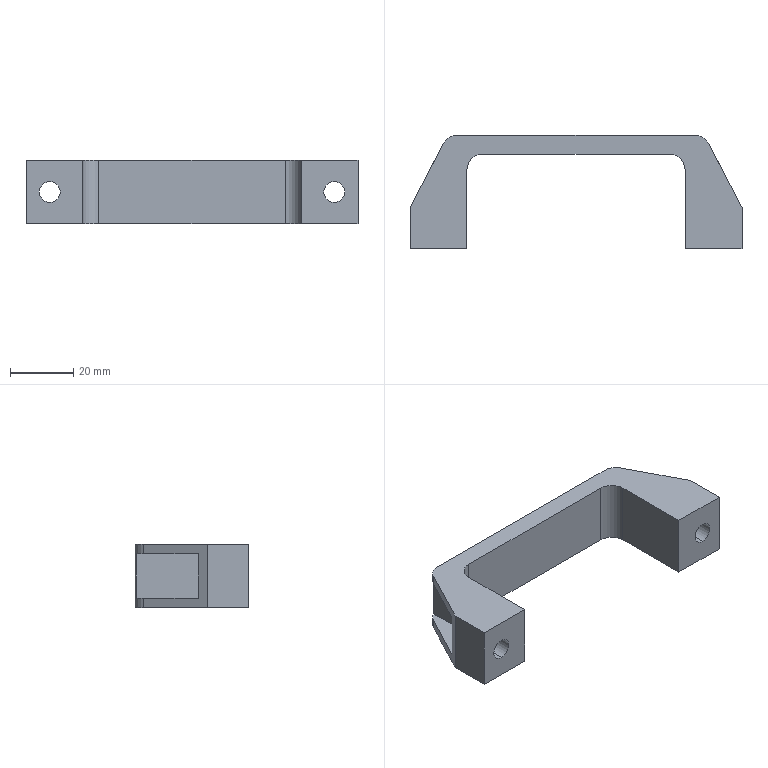Part | SolidWorks | features Fillet 2, Extrusion 1, HoleWzd 1, ICE 1 | 1 solid | 38 faces | box 105 x 36 x 20 mm | volume 23720 mm3 | plane 22 | cylinder 12 | cone 4 | commonest cylinder face diameters 6.6 x4 10 x4 11 x4
STEP:
#1=CARTESIAN_POINT('',(-36.648,0.4785,4.5));
#2=VERTEX_POINT('',#1);
#3=CARTESIAN_POINT('',(-36.648,0.4785,15.5));
#4=VERTEX_POINT('',#3);
#5=CARTESIAN_POINT('',(-36.648,0.4785,10.));
#6=DIRECTION('',(0.,1.,0.));
#7=DIRECTION('',(0.,0.,1.));
#8=AXIS2_PLACEMENT_3D('',#5,#6,#7);
#9=CIRCLE('',#8,5.5);
#10=EDGE_CURVE('',#2,#4,#9,.T.);
#11=ORIENTED_EDGE('',*,*,#10,.F.);
#12=CARTESIAN_POINT('',(-36.648,5.178,4.5));
#13=VERTEX_POINT('',#12);
#14=CARTESIAN_POINT('',(-36.648,5.178,4.5));
#15=DIRECTION('',(0.,1.,0.));
#16=VECTOR('',#15,1000.);
#17=LINE('',#14,#16);
#18=EDGE_CURVE('',#2,#13,#17,.T.);
#19=ORIENTED_EDGE('',*,*,#18,.T.);
#20=CARTESIAN_POINT('',(-36.648,5.178,15.5));
#21=VERTEX_POINT('',#20);
#22=CARTESIAN_POINT('',(-36.648,5.178,10.));
#23=DIRECTION('',(0.,1.,0.));
#24=DIRECTION('',(0.,0.,1.));
#25=AXIS2_PLACEMENT_3D('',#22,#23,#24);
#26=CIRCLE('',#25,5.5);
#27=EDGE_CURVE('',#13,#21,#26,.T.);
#28=ORIENTED_EDGE('',*,*,#27,.T.);
#29=CARTESIAN_POINT('',(-36.648,5.178,15.5));
#30=DIRECTION('',(0.,1.,0.));
#31=VECTOR('',#30,1000.);
#32=LINE('',#29,#31);
#33=EDGE_CURVE('',#4,#21,#32,.T.);
#34=ORIENTED_EDGE('',*,*,#33,.F.);
#35=EDGE_LOOP('',(#11,#19,#28,#34));
#36=FACE_OUTER_BOUND('',#35,.T.);
#37=CARTESIAN_POINT('',(-36.648,5.178,10.));
#38=DIRECTION('',(0.,1.,0.));
#39=DIRECTION('',(0.,0.,1.));
#40=AXIS2_PLACEMENT_3D('',#37,#38,#39);
#41=CYLINDRICAL_SURFACE('',#40,5.5);
#42=ADVANCED_FACE('',(#36),#41,.F.);
#43=CARTESIAN_POINT('',(-36.648,0.4535,6.7));
#44=VERTEX_POINT('',#43);
#45=CARTESIAN_POINT('',(-36.648,0.4535,13.3));
#46=VERTEX_POINT('',#45);
#47=CARTESIAN_POINT('',(-36.648,0.4535,10.));
#48=DIRECTION('',(0.,1.,0.));
#49=DIRECTION('',(0.,0.,1.));
#50=AXIS2_PLACEMENT_3D('',#47,#48,#49);
#51=CIRCLE('',#50,3.3);
#52=EDGE_CURVE('',#44,#46,#51,.T.);
#53=ORIENTED_EDGE('',*,*,#52,.F.);
#54=CARTESIAN_POINT('',(-36.648,0.4785,6.675));
#55=VERTEX_POINT('',#54);
#56=CARTESIAN_POINT('',(-36.648,0.4785,6.675));
#57=DIRECTION('',(0.,0.7071,-0.7071));
#58=VECTOR('',#57,1000.);
#59=LINE('',#56,#58);
#60=EDGE_CURVE('',#44,#55,#59,.T.);
#61=ORIENTED_EDGE('',*,*,#60,.T.);
#62=CARTESIAN_POINT('',(-36.648,0.4785,13.325));
#63=VERTEX_POINT('',#62);
#64=CARTESIAN_POINT('',(-36.648,0.4785,10.));
#65=DIRECTION('',(0.,1.,0.));
#66=DIRECTION('',(0.,0.,1.));
#67=AXIS2_PLACEMENT_3D('',#64,#65,#66);
#68=CIRCLE('',#67,3.325);
#69=EDGE_CURVE('',#55,#63,#68,.T.);
#70=ORIENTED_EDGE('',*,*,#69,.T.);
#71=CARTESIAN_POINT('',(-36.648,0.4785,13.325));
#72=DIRECTION('',(0.,0.7071,0.7071));
#73=VECTOR('',#72,1000.);
#74=LINE('',#71,#73);
#75=EDGE_CURVE('',#46,#63,#74,.T.);
#76=ORIENTED_EDGE('',*,*,#75,.F.);
#77=EDGE_LOOP('',(#53,#61,#70,#76));
#78=FACE_OUTER_BOUND('',#77,.T.);
#79=CARTESIAN_POINT('',(-36.648,0.4785,10.));
#80=DIRECTION('',(0.,1.,0.));
#81=DIRECTION('',(0.,0.,1.));
#82=AXIS2_PLACEMENT_3D('',#79,#80,#81);
#83=CONICAL_SURFACE('',#82,3.325,0.7854);
#84=ADVANCED_FACE('',(#78),#83,.F.);
#85=CARTESIAN_POINT('',(-36.648,-10.822,6.7));
#86=VERTEX_POINT('',#85);
#87=CARTESIAN_POINT('',(-36.648,-10.822,13.3));
#88=VERTEX_POINT('',#87);
#89=CARTESIAN_POINT('',(-36.648,-10.822,10.));
#90=DIRECTION('',(0.,1.,0.));
#91=DIRECTION('',(0.,0.,1.));
#92=AXIS2_PLACEMENT_3D('',#89,#90,#91);
#93=CIRCLE('',#92,3.3);
#94=EDGE_CURVE('',#86,#88,#93,.T.);
#95=ORIENTED_EDGE('',*,*,#94,.F.);
#96=CARTESIAN_POINT('',(-36.648,5.178,6.7));
#97=DIRECTION('',(0.,1.,0.));
#98=VECTOR('',#97,1000.);
#99=LINE('',#96,#98);
#100=EDGE_CURVE('',#86,#44,#99,.T.);
#101=ORIENTED_EDGE('',*,*,#100,.T.);
#102=ORIENTED_EDGE('',*,*,#52,.T.);
#103=CARTESIAN_POINT('',(-36.648,5.178,13.3));
#104=DIRECTION('',(0.,1.,0.));
#105=VECTOR('',#104,1000.);
#106=LINE('',#103,#105);
#107=EDGE_CURVE('',#88,#46,#106,.T.);
#108=ORIENTED_EDGE('',*,*,#107,.F.);
#109=EDGE_LOOP('',(#95,#101,#102,#108));
#110=FACE_OUTER_BOUND('',#109,.T.);
#111=CARTESIAN_POINT('',(-36.648,5.178,10.));
#112=DIRECTION('',(0.,1.,0.));
#113=DIRECTION('',(0.,0.,1.));
#114=AXIS2_PLACEMENT_3D('',#111,#112,#113);
#115=CYLINDRICAL_SURFACE('',#114,3.3);
#116=ADVANCED_FACE('',(#110),#115,.F.);
#117=CARTESIAN_POINT('',(53.352,0.4785,4.5));
#118=VERTEX_POINT('',#117);
#119=CARTESIAN_POINT('',(53.352,0.4785,15.5));
#120=VERTEX_POINT('',#119);
#121=CARTESIAN_POINT('',(53.352,0.4785,10.));
#122=DIRECTION('',(0.,1.,0.));
#123=DIRECTION('',(0.,0.,1.));
#124=AXIS2_PLACEMENT_3D('',#121,#122,#123);
#125=CIRCLE('',#124,5.5);
#126=EDGE_CURVE('',#118,#120,#125,.T.);
#127=ORIENTED_EDGE('',*,*,#126,.F.);
#128=CARTESIAN_POINT('',(53.352,5.178,4.5));
#129=VERTEX_POINT('',#128);
#130=CARTESIAN_POINT('',(53.352,5.178,4.5));
#131=DIRECTION('',(0.,1.,0.));
#132=VECTOR('',#131,1000.);
#133=LINE('',#130,#132);
#134=EDGE_CURVE('',#118,#129,#133,.T.);
#135=ORIENTED_EDGE('',*,*,#134,.T.);
#136=CARTESIAN_POINT('',(47.852,5.178,10.));
#137=VERTEX_POINT('',#136);
#138=CARTESIAN_POINT('',(53.352,5.178,10.));
#139=DIRECTION('',(0.,1.,0.));
#140=DIRECTION('',(0.,0.,1.));
#141=AXIS2_PLACEMENT_3D('',#138,#139,#140);
#142=CIRCLE('',#141,5.5);
#143=EDGE_CURVE('',#129,#137,#142,.T.);
#144=ORIENTED_EDGE('',*,*,#143,.T.);
#145=CARTESIAN_POINT('',(53.352,5.178,15.5));
#146=VERTEX_POINT('',#145);
#147=CARTESIAN_POINT('',(53.352,5.178,10.));
#148=DIRECTION('',(0.,1.,0.));
#149=DIRECTION('',(0.,0.,1.));
#150=AXIS2_PLACEMENT_3D('',#147,#148,#149);
#151=CIRCLE('',#150,5.5);
#152=EDGE_CURVE('',#137,#146,#151,.T.);
#153=ORIENTED_EDGE('',*,*,#152,.T.);
#154=CARTESIAN_POINT('',(53.352,5.178,15.5));
#155=DIRECTION('',(0.,1.,0.));
#156=VECTOR('',#155,1000.);
#157=LINE('',#154,#156);
#158=EDGE_CURVE('',#120,#146,#157,.T.);
#159=ORIENTED_EDGE('',*,*,#158,.F.);
#160=EDGE_LOOP('',(#127,#135,#144,#153,#159));
#161=FACE_OUTER_BOUND('',#160,.T.);
#162=CARTESIAN_POINT('',(53.352,5.178,10.));
#163=DIRECTION('',(0.,1.,0.));
#164=DIRECTION('',(0.,0.,1.));
#165=AXIS2_PLACEMENT_3D('',#162,#163,#164);
#166=CYLINDRICAL_SURFACE('',#165,5.5);
#167=ADVANCED_FACE('',(#161),#166,.F.);
#168=CARTESIAN_POINT('',(53.352,0.4535,6.7));
#169=VERTEX_POINT('',#168);
#170=CARTESIAN_POINT('',(53.352,0.4535,13.3));
#171=VERTEX_POINT('',#170);
#172=CARTESIAN_POINT('',(53.352,0.4535,10.));
#173=DIRECTION('',(0.,1.,0.));
#174=DIRECTION('',(0.,0.,1.));
#175=AXIS2_PLACEMENT_3D('',#172,#173,#174);
#176=CIRCLE('',#175,3.3);
#177=EDGE_CURVE('',#169,#171,#176,.T.);
#178=ORIENTED_EDGE('',*,*,#177,.F.);
#179=CARTESIAN_POINT('',(53.352,0.4785,6.675));
#180=VERTEX_POINT('',#179);
#181=CARTESIAN_POINT('',(53.352,0.4785,6.675));
#182=DIRECTION('',(0.,0.7071,-0.7071));
#183=VECTOR('',#182,1000.);
#184=LINE('',#181,#183);
#185=EDGE_CURVE('',#169,#180,#184,.T.);
#186=ORIENTED_EDGE('',*,*,#185,.T.);
#187=CARTESIAN_POINT('',(53.352,0.4785,13.325));
#188=VERTEX_POINT('',#187);
#189=CARTESIAN_POINT('',(53.352,0.4785,10.));
#190=DIRECTION('',(0.,1.,0.));
#191=DIRECTION('',(0.,0.,1.));
#192=AXIS2_PLACEMENT_3D('',#189,#190,#191);
#193=CIRCLE('',#192,3.325);
#194=EDGE_CURVE('',#180,#188,#193,.T.);
#195=ORIENTED_EDGE('',*,*,#194,.T.);
#196=CARTESIAN_POINT('',(53.352,0.4785,13.325));
#197=DIRECTION('',(0.,0.7071,0.7071));
#198=VECTOR('',#197,1000.);
#199=LINE('',#196,#198);
#200=EDGE_CURVE('',#171,#188,#199,.T.);
#201=ORIENTED_EDGE('',*,*,#200,.F.);
#202=EDGE_LOOP('',(#178,#186,#195,#201));
#203=FACE_OUTER_BOUND('',#202,.T.);
#204=CARTESIAN_POINT('',(53.352,0.4785,10.));
#205=DIRECTION('',(0.,1.,0.));
#206=DIRECTION('',(0.,0.,1.));
#207=AXIS2_PLACEMENT_3D('',#204,#205,#206);
#208=CONICAL_SURFACE('',#207,3.325,0.7854);
#209=ADVANCED_FACE('',(#203),#208,.F.);
#210=CARTESIAN_POINT('',(53.352,-10.822,6.7));
#211=VERTEX_POINT('',#210);
#212=CARTESIAN_POINT('',(53.352,-10.822,13.3));
#213=VERTEX_POINT('',#212);
#214=CARTESIAN_POINT('',(53.352,-10.822,10.));
#215=DIRECTION('',(0.,1.,0.));
#216=DIRECTION('',(0.,0.,1.));
#217=AXIS2_PLACEMENT_3D('',#214,#215,#216);
#218=CIRCLE('',#217,3.3);
#219=EDGE_CURVE('',#211,#213,#218,.T.);
#220=ORIENTED_EDGE('',*,*,#219,.F.);
#221=CARTESIAN_POINT('',(53.352,5.178,6.7));
#222=DIRECTION('',(0.,1.,0.));
#223=VECTOR('',#222,1000.);
#224=LINE('',#221,#223);
#225=EDGE_CURVE('',#211,#169,#224,.T.);
#226=ORIENTED_EDGE('',*,*,#225,.T.);
#227=ORIENTED_EDGE('',*,*,#177,.T.);
#228=CARTESIAN_POINT('',(53.352,5.178,13.3));
#229=DIRECTION('',(0.,1.,0.));
#230=VECTOR('',#229,1000.);
#231=LINE('',#228,#230);
#232=EDGE_CURVE('',#213,#171,#231,.T.);
#233=ORIENTED_EDGE('',*,*,#232,.F.);
#234=EDGE_LOOP('',(#220,#226,#227,#233));
#235=FACE_OUTER_BOUND('',#234,.T.);
#236=CARTESIAN_POINT('',(53.352,5.178,10.));
#237=DIRECTION('',(0.,1.,0.));
#238=DIRECTION('',(0.,0.,1.));
#239=AXIS2_PLACEMENT_3D('',#236,#237,#238);
#240=CYLINDRICAL_SURFACE('',#239,3.3);
#241=ADVANCED_FACE('',(#235),#240,.F.);
#242=CARTESIAN_POINT('',(-26.148,-10.822,0.));
#243=VERTEX_POINT('',#242);
#244=CARTESIAN_POINT('',(-26.148,14.178,0.));
#245=VERTEX_POINT('',#244);
#246=CARTESIAN_POINT('',(-26.148,19.178,0.));
#247=DIRECTION('',(0.,1.,0.));
#248=VECTOR('',#247,1000.);
#249=LINE('',#246,#248);
#250=EDGE_CURVE('',#243,#245,#249,.T.);
#251=ORIENTED_EDGE('',*,*,#250,.T.);
#252=CARTESIAN_POINT('',(-26.148,14.178,20.));
#253=VERTEX_POINT('',#252);
#254=CARTESIAN_POINT('',(-26.148,14.178,20.));
#255=DIRECTION('',(0.,0.,1.));
#256=VECTOR('',#255,1000.);
#257=LINE('',#254,#256);
#258=EDGE_CURVE('',#245,#253,#257,.T.);
#259=ORIENTED_EDGE('',*,*,#258,.T.);
#260=CARTESIAN_POINT('',(-26.148,-10.822,20.));
#261=VERTEX_POINT('',#260);
#262=CARTESIAN_POINT('',(-26.148,19.178,20.));
#263=DIRECTION('',(0.,1.,0.));
#264=VECTOR('',#263,1000.);
#265=LINE('',#262,#264);
#266=EDGE_CURVE('',#261,#253,#265,.T.);
#267=ORIENTED_EDGE('',*,*,#266,.F.);
#268=CARTESIAN_POINT('',(-26.148,-10.822,20.));
#269=DIRECTION('',(0.,0.,-1.));
#270=VECTOR('',#269,1000.);
#271=LINE('',#268,#270);
#272=EDGE_CURVE('',#261,#243,#271,.T.);
#273=ORIENTED_EDGE('',*,*,#272,.T.);
#274=EDGE_LOOP('',(#251,#259,#267,#273));
#275=FACE_OUTER_BOUND('',#274,.T.);
#276=CARTESIAN_POINT('',(-26.148,19.178,20.));
#277=DIRECTION('',(-1.,0.,0.));
#278=DIRECTION('',(0.,-1.,0.));
#279=AXIS2_PLACEMENT_3D('',#276,#277,#278);
#280=PLANE('',#279);
#281=ADVANCED_FACE('',(#275),#280,.F.);
#282=CARTESIAN_POINT('',(-21.148,19.178,20.));
#283=VERTEX_POINT('',#282);
#284=CARTESIAN_POINT('',(37.852,19.178,20.));
#285=VERTEX_POINT('',#284);
#286=CARTESIAN_POINT('',(-26.148,19.178,20.));
#287=DIRECTION('',(1.,0.,0.));
#288=VECTOR('',#287,1000.);
#289=LINE('',#286,#288);
#290=EDGE_CURVE('',#283,#285,#289,.T.);
#291=ORIENTED_EDGE('',*,*,#290,.F.);
#292=CARTESIAN_POINT('',(-21.148,19.178,0.));
#293=VERTEX_POINT('',#292);
#294=CARTESIAN_POINT('',(-21.148,19.178,0.));
#295=DIRECTION('',(0.,0.,-1.));
#296=VECTOR('',#295,1000.);
#297=LINE('',#294,#296);
#298=EDGE_CURVE('',#283,#293,#297,.T.);
#299=ORIENTED_EDGE('',*,*,#298,.T.);
#300=CARTESIAN_POINT('',(37.852,19.178,0.));
#301=VERTEX_POINT('',#300);
#302=CARTESIAN_POINT('',(-26.148,19.178,0.));
#303=DIRECTION('',(1.,0.,0.));
#304=VECTOR('',#303,1000.);
#305=LINE('',#302,#304);
#306=EDGE_CURVE('',#293,#301,#305,.T.);
#307=ORIENTED_EDGE('',*,*,#306,.T.);
#308=CARTESIAN_POINT('',(37.852,19.178,20.));
#309=DIRECTION('',(0.,0.,1.));
#310=VECTOR('',#309,1000.);
#311=LINE('',#308,#310);
#312=EDGE_CURVE('',#301,#285,#311,.T.);
#313=ORIENTED_EDGE('',*,*,#312,.T.);
#314=EDGE_LOOP('',(#291,#299,#307,#313));
#315=FACE_OUTER_BOUND('',#314,.T.);
#316=CARTESIAN_POINT('',(-26.148,19.178,20.));
#317=DIRECTION('',(0.,1.,0.));
#318=DIRECTION('',(-1.,0.,0.));
#319=AXIS2_PLACEMENT_3D('',#316,#317,#318);
#320=PLANE('',#319);
#321=ADVANCED_FACE('',(#315),#320,.F.);
#322=CARTESIAN_POINT('',(42.852,14.178,20.));
#323=VERTEX_POINT('',#322);
#324=CARTESIAN_POINT('',(42.852,-10.822,20.));
#325=VERTEX_POINT('',#324);
#326=CARTESIAN_POINT('',(42.852,19.178,20.));
#327=DIRECTION('',(0.,-1.,0.));
#328=VECTOR('',#327,1000.);
#329=LINE('',#326,#328);
#330=EDGE_CURVE('',#323,#325,#329,.T.);
#331=ORIENTED_EDGE('',*,*,#330,.F.);
#332=CARTESIAN_POINT('',(42.852,14.178,0.));
#333=VERTEX_POINT('',#332);
#334=CARTESIAN_POINT('',(42.852,14.178,0.));
#335=DIRECTION('',(0.,0.,-1.));
#336=VECTOR('',#335,1000.);
#337=LINE('',#334,#336);
#338=EDGE_CURVE('',#323,#333,#337,.T.);
#339=ORIENTED_EDGE('',*,*,#338,.T.);
#340=CARTESIAN_POINT('',(42.852,-10.822,0.));
#341=VERTEX_POINT('',#340);
#342=CARTESIAN_POINT('',(42.852,19.178,0.));
#343=DIRECTION('',(0.,-1.,0.));
#344=VECTOR('',#343,1000.);
#345=LINE('',#342,#344);
#346=EDGE_CURVE('',#333,#341,#345,.T.);
#347=ORIENTED_EDGE('',*,*,#346,.T.);
#348=CARTESIAN_POINT('',(42.852,-10.822,20.));
#349=DIRECTION('',(0.,0.,-1.));
#350=VECTOR('',#349,1000.);
#351=LINE('',#348,#350);
#352=EDGE_CURVE('',#325,#341,#351,.T.);
#353=ORIENTED_EDGE('',*,*,#352,.F.);
#354=EDGE_LOOP('',(#331,#339,#347,#353));
#355=FACE_OUTER_BOUND('',#354,.T.);
#356=CARTESIAN_POINT('',(42.852,19.178,20.));
#357=DIRECTION('',(1.,0.,0.));
#358=DIRECTION('',(0.,0.,-1.));
#359=AXIS2_PLACEMENT_3D('',#356,#357,#358);
#360=PLANE('',#359);
#361=ADVANCED_FACE('',(#355),#360,.F.);
#362=CARTESIAN_POINT('',(53.352,-10.822,10.));
#363=DIRECTION('',(0.,1.,0.));
#364=DIRECTION('',(0.,0.,1.));
#365=AXIS2_PLACEMENT_3D('',#362,#363,#364);
#366=CIRCLE('',#365,3.3);
#367=EDGE_CURVE('',#213,#211,#366,.T.);
#368=ORIENTED_EDGE('',*,*,#367,.T.);
#369=ORIENTED_EDGE('',*,*,#219,.T.);
#370=EDGE_LOOP('',(#368,#369));
#371=FACE_BOUND('',#370,.T.);
#372=CARTESIAN_POINT('',(60.852,-10.822,0.));
#373=VERTEX_POINT('',#372);
#374=CARTESIAN_POINT('',(60.852,-10.822,0.));
#375=DIRECTION('',(1.,0.,0.));
#376=VECTOR('',#375,1000.);
#377=LINE('',#374,#376);
#378=EDGE_CURVE('',#341,#373,#377,.T.);
#379=ORIENTED_EDGE('',*,*,#378,.T.);
#380=CARTESIAN_POINT('',(60.852,-10.822,20.));
#381=VERTEX_POINT('',#380);
#382=CARTESIAN_POINT('',(60.852,-10.822,20.));
#383=DIRECTION('',(0.,0.,-1.));
#384=VECTOR('',#383,1000.);
#385=LINE('',#382,#384);
#386=EDGE_CURVE('',#381,#373,#385,.T.);
#387=ORIENTED_EDGE('',*,*,#386,.F.);
#388=CARTESIAN_POINT('',(60.852,-10.822,20.));
#389=DIRECTION('',(1.,0.,0.));
#390=VECTOR('',#389,1000.);
#391=LINE('',#388,#390);
#392=EDGE_CURVE('',#325,#381,#391,.T.);
#393=ORIENTED_EDGE('',*,*,#392,.F.);
#394=ORIENTED_EDGE('',*,*,#352,.T.);
#395=EDGE_LOOP('',(#379,#387,#393,#394));
#396=FACE_OUTER_BOUND('',#395,.T.);
#397=CARTESIAN_POINT('',(60.852,-10.822,20.));
#398=DIRECTION('',(0.,1.,0.));
#399=DIRECTION('',(-1.,0.,0.));
#400=AXIS2_PLACEMENT_3D('',#397,#398,#399);
#401=PLANE('',#400);
#402=ADVANCED_FACE('',(#371,#396),#401,.F.);
#403=CARTESIAN_POINT('',(60.852,2.178,0.));
#404=VERTEX_POINT('',#403);
#405=CARTESIAN_POINT('',(60.852,2.178,0.));
#406=DIRECTION('',(0.,1.,0.));
#407=VECTOR('',#406,1000.);
#408=LINE('',#405,#407);
#409=EDGE_CURVE('',#373,#404,#408,.T.);
#410=ORIENTED_EDGE('',*,*,#409,.T.);
#411=CARTESIAN_POINT('',(60.852,2.178,20.));
#412=VERTEX_POINT('',#411);
#413=CARTESIAN_POINT('',(60.852,2.178,20.));
#414=DIRECTION('',(0.,0.,-1.));
#415=VECTOR('',#414,1000.);
#416=LINE('',#413,#415);
#417=EDGE_CURVE('',#412,#404,#416,.T.);
#418=ORIENTED_EDGE('',*,*,#417,.F.);
#419=CARTESIAN_POINT('',(60.852,2.178,20.));
#420=DIRECTION('',(0.,1.,0.));
#421=VECTOR('',#420,1000.);
#422=LINE('',#419,#421);
#423=EDGE_CURVE('',#381,#412,#422,.T.);
#424=ORIENTED_EDGE('',*,*,#423,.F.);
#425=ORIENTED_EDGE('',*,*,#386,.T.);
#426=EDGE_LOOP('',(#410,#418,#424,#425));
#427=FACE_OUTER_BOUND('',#426,.T.);
#428=CARTESIAN_POINT('',(60.852,2.178,20.));
#429=DIRECTION('',(-1.,0.,0.));
#430=DIRECTION('',(0.,-1.,0.));
#431=AXIS2_PLACEMENT_3D('',#428,#429,#430);
#432=PLANE('',#431);
#433=ADVANCED_FACE('',(#427),#432,.F.);
#434=CARTESIAN_POINT('',(59.287,5.178,17.));
#435=VERTEX_POINT('',#434);
#436=CARTESIAN_POINT('',(50.254,22.491,17.));
#437=VERTEX_POINT('',#436);
#438=CARTESIAN_POINT('',(48.852,25.178,17.));
#439=DIRECTION('',(-0.4626,0.8866,0.));
#440=VECTOR('',#439,1000.);
#441=LINE('',#438,#440);
#442=EDGE_CURVE('',#435,#437,#441,.T.);
#443=ORIENTED_EDGE('',*,*,#442,.T.);
#444=CARTESIAN_POINT('',(50.254,22.491,20.));
#445=VERTEX_POINT('',#444);
#446=CARTESIAN_POINT('',(50.254,22.491,20.));
#447=DIRECTION('',(0.,0.,1.));
#448=VECTOR('',#447,1000.);
#449=LINE('',#446,#448);
#450=EDGE_CURVE('',#437,#445,#449,.T.);
#451=ORIENTED_EDGE('',*,*,#450,.T.);
#452=CARTESIAN_POINT('',(48.852,25.178,20.));
#453=DIRECTION('',(-0.4626,0.8866,0.));
#454=VECTOR('',#453,1000.);
#455=LINE('',#452,#454);
#456=EDGE_CURVE('',#412,#445,#455,.T.);
#457=ORIENTED_EDGE('',*,*,#456,.F.);
#458=ORIENTED_EDGE('',*,*,#417,.T.);
#459=CARTESIAN_POINT('',(50.254,22.491,0.));
#460=VERTEX_POINT('',#459);
#461=CARTESIAN_POINT('',(48.852,25.178,0.));
#462=DIRECTION('',(-0.4626,0.8866,0.));
#463=VECTOR('',#462,1000.);
#464=LINE('',#461,#463);
#465=EDGE_CURVE('',#404,#460,#464,.T.);
#466=ORIENTED_EDGE('',*,*,#465,.T.);
#467=CARTESIAN_POINT('',(50.254,22.491,3.));
#468=VERTEX_POINT('',#467);
#469=CARTESIAN_POINT('',(50.254,22.491,20.));
#470=DIRECTION('',(0.,0.,1.));
#471=VECTOR('',#470,1000.);
#472=LINE('',#469,#471);
#473=EDGE_CURVE('',#460,#468,#472,.T.);
#474=ORIENTED_EDGE('',*,*,#473,.T.);
#475=CARTESIAN_POINT('',(59.287,5.178,3.));
#476=VERTEX_POINT('',#475);
#477=CARTESIAN_POINT('',(48.852,25.178,3.));
#478=DIRECTION('',(0.4626,-0.8866,0.));
#479=VECTOR('',#478,1000.);
#480=LINE('',#477,#479);
#481=EDGE_CURVE('',#468,#476,#480,.T.);
#482=ORIENTED_EDGE('',*,*,#481,.T.);
#483=CARTESIAN_POINT('',(59.287,5.178,20.));
#484=DIRECTION('',(0.,0.,-1.));
#485=VECTOR('',#484,1000.);
#486=LINE('',#483,#485);
#487=EDGE_CURVE('',#435,#476,#486,.T.);
#488=ORIENTED_EDGE('',*,*,#487,.F.);
#489=EDGE_LOOP('',(#443,#451,#457,#458,#466,#474,#482,#488));
#490=FACE_OUTER_BOUND('',#489,.T.);
#491=CARTESIAN_POINT('',(48.852,25.178,20.));
#492=DIRECTION('',(-0.8866,-0.4626,0.));
#493=DIRECTION('',(0.4626,-0.8866,0.));
#494=AXIS2_PLACEMENT_3D('',#491,#492,#493);
#495=PLANE('',#494);
#496=ADVANCED_FACE('',(#490),#495,.F.);
#497=CARTESIAN_POINT('',(45.821,25.178,20.));
#498=VERTEX_POINT('',#497);
#499=CARTESIAN_POINT('',(-29.117,25.178,20.));
#500=VERTEX_POINT('',#499);
#501=CARTESIAN_POINT('',(48.852,25.178,20.));
#502=DIRECTION('',(-1.,0.,0.));
#503=VECTOR('',#502,1000.);
#504=LINE('',#501,#503);
#505=EDGE_CURVE('',#498,#500,#504,.T.);
#506=ORIENTED_EDGE('',*,*,#505,.F.);
#507=CARTESIAN_POINT('',(45.821,25.178,0.));
#508=VERTEX_POINT('',#507);
#509=CARTESIAN_POINT('',(45.821,25.178,20.));
#510=DIRECTION('',(0.,0.,-1.));
#511=VECTOR('',#510,1000.);
#512=LINE('',#509,#511);
#513=EDGE_CURVE('',#498,#508,#512,.T.);
#514=ORIENTED_EDGE('',*,*,#513,.T.);
#515=CARTESIAN_POINT('',(-29.117,25.178,0.));
#516=VERTEX_POINT('',#515);
#517=CARTESIAN_POINT('',(48.852,25.178,0.));
#518=DIRECTION('',(-1.,0.,0.));
#519=VECTOR('',#518,1000.);
#520=LINE('',#517,#519);
#521=EDGE_CURVE('',#508,#516,#520,.T.);
#522=ORIENTED_EDGE('',*,*,#521,.T.);
#523=CARTESIAN_POINT('',(-29.117,25.178,20.));
#524=DIRECTION('',(0.,0.,1.));
#525=VECTOR('',#524,1000.);
#526=LINE('',#523,#525);
#527=EDGE_CURVE('',#516,#500,#526,.T.);
#528=ORIENTED_EDGE('',*,*,#527,.T.);
#529=EDGE_LOOP('',(#506,#514,#522,#528));
#530=FACE_OUTER_BOUND('',#529,.T.);
#531=CARTESIAN_POINT('',(48.852,25.178,20.));
#532=DIRECTION('',(0.,-1.,0.));
#533=DIRECTION('',(1.,0.,0.));
#534=AXIS2_PLACEMENT_3D('',#531,#532,#533);
#535=PLANE('',#534);
#536=ADVANCED_FACE('',(#530),#535,.F.);
#537=CARTESIAN_POINT('',(-33.55,22.491,20.));
#538=VERTEX_POINT('',#537);
#539=CARTESIAN_POINT('',(-44.148,2.178,20.));
#540=VERTEX_POINT('',#539);
#541=CARTESIAN_POINT('',(-32.148,25.178,20.));
#542=DIRECTION('',(-0.4626,-0.8866,0.));
#543=VECTOR('',#542,1000.);
#544=LINE('',#541,#543);
#545=EDGE_CURVE('',#538,#540,#544,.T.);
#546=ORIENTED_EDGE('',*,*,#545,.F.);
#547=CARTESIAN_POINT('',(-33.55,22.491,17.));
#548=VERTEX_POINT('',#547);
#549=CARTESIAN_POINT('',(-33.55,22.491,20.));
#550=DIRECTION('',(0.,0.,-1.));
#551=VECTOR('',#550,1000.);
#552=LINE('',#549,#551);
#553=EDGE_CURVE('',#538,#548,#552,.T.);
#554=ORIENTED_EDGE('',*,*,#553,.T.);
#555=CARTESIAN_POINT('',(-42.583,5.178,17.));
#556=VERTEX_POINT('',#555);
#557=CARTESIAN_POINT('',(-32.148,25.178,17.));
#558=DIRECTION('',(-0.4626,-0.8866,0.));
#559=VECTOR('',#558,1000.);
#560=LINE('',#557,#559);
#561=EDGE_CURVE('',#548,#556,#560,.T.);
#562=ORIENTED_EDGE('',*,*,#561,.T.);
#563=CARTESIAN_POINT('',(-42.583,5.178,3.));
#564=VERTEX_POINT('',#563);
#565=CARTESIAN_POINT('',(-42.583,5.178,20.));
#566=DIRECTION('',(0.,0.,1.));
#567=VECTOR('',#566,1000.);
#568=LINE('',#565,#567);
#569=EDGE_CURVE('',#564,#556,#568,.T.);
#570=ORIENTED_EDGE('',*,*,#569,.F.);
#571=CARTESIAN_POINT('',(-33.55,22.491,3.));
#572=VERTEX_POINT('',#571);
#573=CARTESIAN_POINT('',(-32.148,25.178,3.));
#574=DIRECTION('',(0.4626,0.8866,0.));
#575=VECTOR('',#574,1000.);
#576=LINE('',#573,#575);
#577=EDGE_CURVE('',#564,#572,#576,.T.);
#578=ORIENTED_EDGE('',*,*,#577,.T.);
#579=CARTESIAN_POINT('',(-33.55,22.491,0.));
#580=VERTEX_POINT('',#579);
#581=CARTESIAN_POINT('',(-33.55,22.491,20.));
#582=DIRECTION('',(0.,0.,-1.));
#583=VECTOR('',#582,1000.);
#584=LINE('',#581,#583);
#585=EDGE_CURVE('',#572,#580,#584,.T.);
#586=ORIENTED_EDGE('',*,*,#585,.T.);
#587=CARTESIAN_POINT('',(-44.148,2.178,0.));
#588=VERTEX_POINT('',#587);
#589=CARTESIAN_POINT('',(-32.148,25.178,0.));
#590=DIRECTION('',(-0.4626,-0.8866,0.));
#591=VECTOR('',#590,1000.);
#592=LINE('',#589,#591);
#593=EDGE_CURVE('',#580,#588,#592,.T.);
#594=ORIENTED_EDGE('',*,*,#593,.T.);
#595=CARTESIAN_POINT('',(-44.148,2.178,20.));
#596=DIRECTION('',(0.,0.,-1.));
#597=VECTOR('',#596,1000.);
#598=LINE('',#595,#597);
#599=EDGE_CURVE('',#540,#588,#598,.T.);
#600=ORIENTED_EDGE('',*,*,#599,.F.);
#601=EDGE_LOOP('',(#546,#554,#562,#570,#578,#586,#594,#600));
#602=FACE_OUTER_BOUND('',#601,.T.);
#603=CARTESIAN_POINT('',(-32.148,25.178,20.));
#604=DIRECTION('',(0.8866,-0.4626,0.));
#605=DIRECTION('',(0.4626,0.8866,0.));
#606=AXIS2_PLACEMENT_3D('',#603,#604,#605);
#607=PLANE('',#606);
#608=ADVANCED_FACE('',(#602),#607,.F.);
#609=CARTESIAN_POINT('',(-44.148,-10.822,0.));
#610=VERTEX_POINT('',#609);
#611=CARTESIAN_POINT('',(-44.148,2.178,0.));
#612=DIRECTION('',(0.,-1.,0.));
#613=VECTOR('',#612,1000.);
#614=LINE('',#611,#613);
#615=EDGE_CURVE('',#588,#610,#614,.T.);
#616=ORIENTED_EDGE('',*,*,#615,.T.);
#617=CARTESIAN_POINT('',(-44.148,-10.822,20.));
#618=VERTEX_POINT('',#617);
#619=CARTESIAN_POINT('',(-44.148,-10.822,20.));
#620=DIRECTION('',(0.,0.,-1.));
#621=VECTOR('',#620,1000.);
#622=LINE('',#619,#621);
#623=EDGE_CURVE('',#618,#610,#622,.T.);
#624=ORIENTED_EDGE('',*,*,#623,.F.);
#625=CARTESIAN_POINT('',(-44.148,2.178,20.));
#626=DIRECTION('',(0.,-1.,0.));
#627=VECTOR('',#626,1000.);
#628=LINE('',#625,#627);
#629=EDGE_CURVE('',#540,#618,#628,.T.);
#630=ORIENTED_EDGE('',*,*,#629,.F.);
#631=ORIENTED_EDGE('',*,*,#599,.T.);
#632=EDGE_LOOP('',(#616,#624,#630,#631));
#633=FACE_OUTER_BOUND('',#632,.T.);
#634=CARTESIAN_POINT('',(-44.148,2.178,20.));
#635=DIRECTION('',(1.,0.,0.));
#636=DIRECTION('',(0.,1.,0.));
#637=AXIS2_PLACEMENT_3D('',#634,#635,#636);
#638=PLANE('',#637);
#639=ADVANCED_FACE('',(#633),#638,.F.);
#640=CARTESIAN_POINT('',(-36.648,-10.822,10.));
#641=DIRECTION('',(0.,1.,0.));
#642=DIRECTION('',(0.,0.,1.));
#643=AXIS2_PLACEMENT_3D('',#640,#641,#642);
#644=CIRCLE('',#643,3.3);
#645=EDGE_CURVE('',#88,#86,#644,.T.);
#646=ORIENTED_EDGE('',*,*,#645,.T.);
#647=ORIENTED_EDGE('',*,*,#94,.T.);
#648=EDGE_LOOP('',(#646,#647));
#649=FACE_BOUND('',#648,.T.);
#650=CARTESIAN_POINT('',(-44.148,-10.822,0.));
#651=DIRECTION('',(1.,0.,0.));
#652=VECTOR('',#651,1000.);
#653=LINE('',#650,#652);
#654=EDGE_CURVE('',#610,#243,#653,.T.);
#655=ORIENTED_EDGE('',*,*,#654,.T.);
#656=ORIENTED_EDGE('',*,*,#272,.F.);
#657=CARTESIAN_POINT('',(-44.148,-10.822,20.));
#658=DIRECTION('',(1.,0.,0.));
#659=VECTOR('',#658,1000.);
#660=LINE('',#657,#659);
#661=EDGE_CURVE('',#618,#261,#660,.T.);
#662=ORIENTED_EDGE('',*,*,#661,.F.);
#663=ORIENTED_EDGE('',*,*,#623,.T.);
#664=EDGE_LOOP('',(#655,#656,#662,#663));
#665=FACE_OUTER_BOUND('',#664,.T.);
#666=CARTESIAN_POINT('',(-44.148,-10.822,20.));
#667=DIRECTION('',(0.,1.,0.));
#668=DIRECTION('',(0.,0.,1.));
#669=AXIS2_PLACEMENT_3D('',#666,#667,#668);
#670=PLANE('',#669);
#671=ADVANCED_FACE('',(#649,#665),#670,.F.);
#672=ORIENTED_EDGE('',*,*,#456,.T.);
#673=CARTESIAN_POINT('',(45.821,20.178,20.));
#674=DIRECTION('',(0.,0.,1.));
#675=DIRECTION('',(1.,0.,0.));
#676=AXIS2_PLACEMENT_3D('',#673,#674,#675);
#677=CIRCLE('',#676,5.);
#678=EDGE_CURVE('',#445,#498,#677,.T.);
#679=ORIENTED_EDGE('',*,*,#678,.T.);
#680=ORIENTED_EDGE('',*,*,#505,.T.);
#681=CARTESIAN_POINT('',(-29.117,20.178,20.));
#682=DIRECTION('',(0.,0.,1.));
#683=DIRECTION('',(1.,0.,0.));
#684=AXIS2_PLACEMENT_3D('',#681,#682,#683);
#685=CIRCLE('',#684,5.);
#686=EDGE_CURVE('',#500,#538,#685,.T.);
#687=ORIENTED_EDGE('',*,*,#686,.T.);
#688=ORIENTED_EDGE('',*,*,#545,.T.);
#689=ORIENTED_EDGE('',*,*,#629,.T.);
#690=ORIENTED_EDGE('',*,*,#661,.T.);
#691=ORIENTED_EDGE('',*,*,#266,.T.);
#692=CARTESIAN_POINT('',(-21.148,14.178,20.));
#693=DIRECTION('',(0.,0.,-1.));
#694=DIRECTION('',(1.,0.,0.));
#695=AXIS2_PLACEMENT_3D('',#692,#693,#694);
#696=CIRCLE('',#695,5.);
#697=EDGE_CURVE('',#253,#283,#696,.T.);
#698=ORIENTED_EDGE('',*,*,#697,.T.);
#699=ORIENTED_EDGE('',*,*,#290,.T.);
#700=CARTESIAN_POINT('',(37.852,14.178,20.));
#701=DIRECTION('',(0.,0.,-1.));
#702=DIRECTION('',(1.,0.,0.));
#703=AXIS2_PLACEMENT_3D('',#700,#701,#702);
#704=CIRCLE('',#703,5.);
#705=EDGE_CURVE('',#285,#323,#704,.T.);
#706=ORIENTED_EDGE('',*,*,#705,.T.);
#707=ORIENTED_EDGE('',*,*,#330,.T.);
#708=ORIENTED_EDGE('',*,*,#392,.T.);
#709=ORIENTED_EDGE('',*,*,#423,.T.);
#710=EDGE_LOOP('',(#672,#679,#680,#687,#688,#689,#690,#691,#698,#699,#706,#707,#708,#709));
#711=FACE_OUTER_BOUND('',#710,.T.);
#712=CARTESIAN_POINT('',(0.,0.,20.));
#713=DIRECTION('',(0.,0.,1.));
#714=DIRECTION('',(1.,0.,0.));
#715=AXIS2_PLACEMENT_3D('',#712,#713,#714);
#716=PLANE('',#715);
#717=ADVANCED_FACE('',(#711),#716,.T.);
#718=ORIENTED_EDGE('',*,*,#521,.F.);
#719=CARTESIAN_POINT('',(45.821,20.178,0.));
#720=DIRECTION('',(0.,0.,-1.));
#721=DIRECTION('',(1.,0.,0.));
#722=AXIS2_PLACEMENT_3D('',#719,#720,#721);
#723=CIRCLE('',#722,5.);
#724=EDGE_CURVE('',#508,#460,#723,.T.);
#725=ORIENTED_EDGE('',*,*,#724,.T.);
#726=ORIENTED_EDGE('',*,*,#465,.F.);
#727=ORIENTED_EDGE('',*,*,#409,.F.);
#728=ORIENTED_EDGE('',*,*,#378,.F.);
#729=ORIENTED_EDGE('',*,*,#346,.F.);
#730=CARTESIAN_POINT('',(37.852,14.178,0.));
#731=DIRECTION('',(0.,0.,1.));
#732=DIRECTION('',(1.,0.,0.));
#733=AXIS2_PLACEMENT_3D('',#730,#731,#732);
#734=CIRCLE('',#733,5.);
#735=EDGE_CURVE('',#333,#301,#734,.T.);
#736=ORIENTED_EDGE('',*,*,#735,.T.);
#737=ORIENTED_EDGE('',*,*,#306,.F.);
#738=CARTESIAN_POINT('',(-21.148,14.178,0.));
#739=DIRECTION('',(0.,0.,1.));
#740=DIRECTION('',(1.,0.,0.));
#741=AXIS2_PLACEMENT_3D('',#738,#739,#740);
#742=CIRCLE('',#741,5.);
#743=EDGE_CURVE('',#293,#245,#742,.T.);
#744=ORIENTED_EDGE('',*,*,#743,.T.);
#745=ORIENTED_EDGE('',*,*,#250,.F.);
#746=ORIENTED_EDGE('',*,*,#654,.F.);
#747=ORIENTED_EDGE('',*,*,#615,.F.);
#748=ORIENTED_EDGE('',*,*,#593,.F.);
#749=CARTESIAN_POINT('',(-29.117,20.178,0.));
#750=DIRECTION('',(0.,0.,-1.));
#751=DIRECTION('',(1.,0.,0.));
#752=AXIS2_PLACEMENT_3D('',#749,#750,#751);
#753=CIRCLE('',#752,5.);
#754=EDGE_CURVE('',#580,#516,#753,.T.);
#755=ORIENTED_EDGE('',*,*,#754,.T.);
#756=EDGE_LOOP('',(#718,#725,#726,#727,#728,#729,#736,#737,#744,#745,#746,#747,#748,#755));
#757=FACE_OUTER_BOUND('',#756,.T.);
#758=CARTESIAN_POINT('',(0.,0.,0.));
#759=DIRECTION('',(0.,0.,1.));
#760=DIRECTION('',(1.,0.,0.));
#761=AXIS2_PLACEMENT_3D('',#758,#759,#760);
#762=PLANE('',#761);
#763=ADVANCED_FACE('',(#757),#762,.F.);
#764=CARTESIAN_POINT('',(-31.148,5.178,3.));
#765=VERTEX_POINT('',#764);
#766=CARTESIAN_POINT('',(-31.148,24.747,3.));
#767=VERTEX_POINT('',#766);
#768=CARTESIAN_POINT('',(-31.148,5.178,3.));
#769=DIRECTION('',(0.,1.,0.));
#770=VECTOR('',#769,1000.);
#771=LINE('',#768,#770);
#772=EDGE_CURVE('',#765,#767,#771,.T.);
#773=ORIENTED_EDGE('',*,*,#772,.T.);
#774=CARTESIAN_POINT('',(-29.117,20.178,3.));
#775=DIRECTION('',(0.,0.,1.));
#776=DIRECTION('',(-1.,0.,0.));
#777=AXIS2_PLACEMENT_3D('',#774,#775,#776);
#778=CIRCLE('',#777,5.);
#779=EDGE_CURVE('',#767,#572,#778,.T.);
#780=ORIENTED_EDGE('',*,*,#779,.T.);
#781=ORIENTED_EDGE('',*,*,#577,.F.);
#782=CARTESIAN_POINT('',(-60.316,5.178,3.));
#783=DIRECTION('',(-1.,0.,0.));
#784=VECTOR('',#783,1000.);
#785=LINE('',#782,#784);
#786=EDGE_CURVE('',#765,#564,#785,.T.);
#787=ORIENTED_EDGE('',*,*,#786,.F.);
#788=EDGE_LOOP('',(#773,#780,#781,#787));
#789=FACE_OUTER_BOUND('',#788,.T.);
#790=CARTESIAN_POINT('',(-60.316,5.178,3.));
#791=DIRECTION('',(0.,0.,-1.));
#792=DIRECTION('',(-1.,0.,0.));
#793=AXIS2_PLACEMENT_3D('',#790,#791,#792);
#794=PLANE('',#793);
#795=ADVANCED_FACE('',(#789),#794,.F.);
#796=ORIENTED_EDGE('',*,*,#561,.F.);
#797=CARTESIAN_POINT('',(-31.148,24.747,17.));
#798=VERTEX_POINT('',#797);
#799=CARTESIAN_POINT('',(-29.117,20.178,17.));
#800=DIRECTION('',(0.,0.,-1.));
#801=DIRECTION('',(1.,0.,0.));
#802=AXIS2_PLACEMENT_3D('',#799,#800,#801);
#803=CIRCLE('',#802,5.);
#804=EDGE_CURVE('',#548,#798,#803,.T.);
#805=ORIENTED_EDGE('',*,*,#804,.T.);
#806=CARTESIAN_POINT('',(-31.148,5.178,17.));
#807=VERTEX_POINT('',#806);
#808=CARTESIAN_POINT('',(-31.148,5.178,17.));
#809=DIRECTION('',(0.,1.,0.));
#810=VECTOR('',#809,1000.);
#811=LINE('',#808,#810);
#812=EDGE_CURVE('',#807,#798,#811,.T.);
#813=ORIENTED_EDGE('',*,*,#812,.F.);
#814=CARTESIAN_POINT('',(-60.316,5.178,17.));
#815=DIRECTION('',(1.,0.,0.));
#816=VECTOR('',#815,1000.);
#817=LINE('',#814,#816);
#818=EDGE_CURVE('',#556,#807,#817,.T.);
#819=ORIENTED_EDGE('',*,*,#818,.F.);
#820=EDGE_LOOP('',(#796,#805,#813,#819));
#821=FACE_OUTER_BOUND('',#820,.T.);
#822=CARTESIAN_POINT('',(-60.316,5.178,17.));
#823=DIRECTION('',(0.,0.,1.));
#824=DIRECTION('',(1.,0.,0.));
#825=AXIS2_PLACEMENT_3D('',#822,#823,#824);
#826=PLANE('',#825);
#827=ADVANCED_FACE('',(#821),#826,.F.);
#828=CARTESIAN_POINT('',(-31.148,5.178,10.));
#829=VERTEX_POINT('',#828);
#830=CARTESIAN_POINT('',(-31.148,5.178,3.));
#831=DIRECTION('',(0.,0.,-1.));
#832=VECTOR('',#831,1000.);
#833=LINE('',#830,#832);
#834=EDGE_CURVE('',#807,#829,#833,.T.);
#835=ORIENTED_EDGE('',*,*,#834,.T.);
#836=CARTESIAN_POINT('',(-36.648,5.178,10.));
#837=DIRECTION('',(0.,1.,0.));
#838=DIRECTION('',(0.,0.,1.));
#839=AXIS2_PLACEMENT_3D('',#836,#837,#838);
#840=CIRCLE('',#839,5.5);
#841=EDGE_CURVE('',#21,#829,#840,.T.);
#842=ORIENTED_EDGE('',*,*,#841,.F.);
#843=ORIENTED_EDGE('',*,*,#27,.F.);
#844=CARTESIAN_POINT('',(-36.648,5.178,10.));
#845=DIRECTION('',(0.,1.,0.));
#846=DIRECTION('',(0.,0.,1.));
#847=AXIS2_PLACEMENT_3D('',#844,#845,#846);
#848=CIRCLE('',#847,5.5);
#849=EDGE_CURVE('',#829,#13,#848,.T.);
#850=ORIENTED_EDGE('',*,*,#849,.F.);
#851=CARTESIAN_POINT('',(-31.148,5.178,3.));
#852=DIRECTION('',(0.,0.,-1.));
#853=VECTOR('',#852,1000.);
#854=LINE('',#851,#853);
#855=EDGE_CURVE('',#829,#765,#854,.T.);
#856=ORIENTED_EDGE('',*,*,#855,.T.);
#857=ORIENTED_EDGE('',*,*,#786,.T.);
#858=ORIENTED_EDGE('',*,*,#569,.T.);
#859=ORIENTED_EDGE('',*,*,#818,.T.);
#860=EDGE_LOOP('',(#835,#842,#843,#850,#856,#857,#858,#859));
#861=FACE_OUTER_BOUND('',#860,.T.);
#862=CARTESIAN_POINT('',(0.,5.178,0.));
#863=DIRECTION('',(0.,1.,0.));
#864=DIRECTION('',(0.,0.,1.));
#865=AXIS2_PLACEMENT_3D('',#862,#863,#864);
#866=PLANE('',#865);
#867=ADVANCED_FACE('',(#861),#866,.T.);
#868=ORIENTED_EDGE('',*,*,#812,.T.);
#869=CARTESIAN_POINT('',(-31.148,24.747,17.));
#870=DIRECTION('',(0.,0.,-1.));
#871=VECTOR('',#870,1000.);
#872=LINE('',#869,#871);
#873=EDGE_CURVE('',#798,#767,#872,.T.);
#874=ORIENTED_EDGE('',*,*,#873,.T.);
#875=ORIENTED_EDGE('',*,*,#772,.F.);
#876=ORIENTED_EDGE('',*,*,#855,.F.);
#877=ORIENTED_EDGE('',*,*,#834,.F.);
#878=EDGE_LOOP('',(#868,#874,#875,#876,#877));
#879=FACE_OUTER_BOUND('',#878,.T.);
#880=CARTESIAN_POINT('',(-31.148,5.178,3.));
#881=DIRECTION('',(1.,0.,0.));
#882=DIRECTION('',(0.,0.,-1.));
#883=AXIS2_PLACEMENT_3D('',#880,#881,#882);
#884=PLANE('',#883);
#885=ADVANCED_FACE('',(#879),#884,.F.);
#886=CARTESIAN_POINT('',(47.852,5.178,3.));
#887=VERTEX_POINT('',#886);
#888=CARTESIAN_POINT('',(47.852,5.178,3.));
#889=DIRECTION('',(0.,0.,1.));
#890=VECTOR('',#889,1000.);
#891=LINE('',#888,#890);
#892=EDGE_CURVE('',#887,#137,#891,.T.);
#893=ORIENTED_EDGE('',*,*,#892,.T.);
#894=ORIENTED_EDGE('',*,*,#143,.F.);
#895=CARTESIAN_POINT('',(53.352,5.178,10.));
#896=DIRECTION('',(0.,1.,0.));
#897=DIRECTION('',(0.,0.,1.));
#898=AXIS2_PLACEMENT_3D('',#895,#896,#897);
#899=CIRCLE('',#898,5.5);
#900=EDGE_CURVE('',#146,#129,#899,.T.);
#901=ORIENTED_EDGE('',*,*,#900,.F.);
#902=ORIENTED_EDGE('',*,*,#152,.F.);
#903=CARTESIAN_POINT('',(47.852,5.178,17.));
#904=VERTEX_POINT('',#903);
#905=CARTESIAN_POINT('',(47.852,5.178,3.));
#906=DIRECTION('',(0.,0.,1.));
#907=VECTOR('',#906,1000.);
#908=LINE('',#905,#907);
#909=EDGE_CURVE('',#137,#904,#908,.T.);
#910=ORIENTED_EDGE('',*,*,#909,.T.);
#911=CARTESIAN_POINT('',(77.02,5.178,17.));
#912=DIRECTION('',(1.,0.,0.));
#913=VECTOR('',#912,1000.);
#914=LINE('',#911,#913);
#915=EDGE_CURVE('',#904,#435,#914,.T.);
#916=ORIENTED_EDGE('',*,*,#915,.T.);
#917=ORIENTED_EDGE('',*,*,#487,.T.);
#918=CARTESIAN_POINT('',(77.02,5.178,3.));
#919=DIRECTION('',(-1.,0.,0.));
#920=VECTOR('',#919,1000.);
#921=LINE('',#918,#920);
#922=EDGE_CURVE('',#476,#887,#921,.T.);
#923=ORIENTED_EDGE('',*,*,#922,.T.);
#924=EDGE_LOOP('',(#893,#894,#901,#902,#910,#916,#917,#923));
#925=FACE_OUTER_BOUND('',#924,.T.);
#926=CARTESIAN_POINT('',(0.,5.178,0.));
#927=DIRECTION('',(0.,1.,0.));
#928=DIRECTION('',(0.,0.,1.));
#929=AXIS2_PLACEMENT_3D('',#926,#927,#928);
#930=PLANE('',#929);
#931=ADVANCED_FACE('',(#925),#930,.T.);
#932=ORIENTED_EDGE('',*,*,#481,.F.);
#933=CARTESIAN_POINT('',(47.852,24.747,3.));
#934=VERTEX_POINT('',#933);
#935=CARTESIAN_POINT('',(45.821,20.178,3.));
#936=DIRECTION('',(0.,0.,1.));
#937=DIRECTION('',(-1.,0.,0.));
#938=AXIS2_PLACEMENT_3D('',#935,#936,#937);
#939=CIRCLE('',#938,5.);
#940=EDGE_CURVE('',#468,#934,#939,.T.);
#941=ORIENTED_EDGE('',*,*,#940,.T.);
#942=CARTESIAN_POINT('',(47.852,5.178,3.));
#943=DIRECTION('',(0.,1.,0.));
#944=VECTOR('',#943,1000.);
#945=LINE('',#942,#944);
#946=EDGE_CURVE('',#887,#934,#945,.T.);
#947=ORIENTED_EDGE('',*,*,#946,.F.);
#948=ORIENTED_EDGE('',*,*,#922,.F.);
#949=EDGE_LOOP('',(#932,#941,#947,#948));
#950=FACE_OUTER_BOUND('',#949,.T.);
#951=CARTESIAN_POINT('',(77.02,5.178,3.));
#952=DIRECTION('',(0.,0.,-1.));
#953=DIRECTION('',(-1.,0.,0.));
#954=AXIS2_PLACEMENT_3D('',#951,#952,#953);
#955=PLANE('',#954);
#956=ADVANCED_FACE('',(#950),#955,.F.);
#957=CARTESIAN_POINT('',(47.852,24.747,17.));
#958=VERTEX_POINT('',#957);
#959=CARTESIAN_POINT('',(47.852,5.178,17.));
#960=DIRECTION('',(0.,1.,0.));
#961=VECTOR('',#960,1000.);
#962=LINE('',#959,#961);
#963=EDGE_CURVE('',#904,#958,#962,.T.);
#964=ORIENTED_EDGE('',*,*,#963,.T.);
#965=CARTESIAN_POINT('',(45.821,20.178,17.));
#966=DIRECTION('',(0.,0.,-1.));
#967=DIRECTION('',(1.,0.,0.));
#968=AXIS2_PLACEMENT_3D('',#965,#966,#967);
#969=CIRCLE('',#968,5.);
#970=EDGE_CURVE('',#958,#437,#969,.T.);
#971=ORIENTED_EDGE('',*,*,#970,.T.);
#972=ORIENTED_EDGE('',*,*,#442,.F.);
#973=ORIENTED_EDGE('',*,*,#915,.F.);
#974=EDGE_LOOP('',(#964,#971,#972,#973));
#975=FACE_OUTER_BOUND('',#974,.T.);
#976=CARTESIAN_POINT('',(77.02,5.178,17.));
#977=DIRECTION('',(0.,0.,1.));
#978=DIRECTION('',(1.,0.,0.));
#979=AXIS2_PLACEMENT_3D('',#976,#977,#978);
#980=PLANE('',#979);
#981=ADVANCED_FACE('',(#975),#980,.F.);
#982=CARTESIAN_POINT('',(47.852,24.747,3.));
#983=DIRECTION('',(0.,0.,1.));
#984=VECTOR('',#983,1000.);
#985=LINE('',#982,#984);
#986=EDGE_CURVE('',#934,#958,#985,.T.);
#987=ORIENTED_EDGE('',*,*,#986,.T.);
#988=ORIENTED_EDGE('',*,*,#963,.F.);
#989=ORIENTED_EDGE('',*,*,#909,.F.);
#990=ORIENTED_EDGE('',*,*,#892,.F.);
#991=ORIENTED_EDGE('',*,*,#946,.T.);
#992=EDGE_LOOP('',(#987,#988,#989,#990,#991));
#993=FACE_OUTER_BOUND('',#992,.T.);
#994=CARTESIAN_POINT('',(47.852,5.178,3.));
#995=DIRECTION('',(-1.,0.,0.));
#996=DIRECTION('',(0.,0.,1.));
#997=AXIS2_PLACEMENT_3D('',#994,#995,#996);
#998=PLANE('',#997);
#999=ADVANCED_FACE('',(#993),#998,.F.);
#1000=ORIENTED_EDGE('',*,*,#225,.F.);
#1001=ORIENTED_EDGE('',*,*,#367,.F.);
#1002=ORIENTED_EDGE('',*,*,#232,.T.);
#1003=CARTESIAN_POINT('',(53.352,0.4535,10.));
#1004=DIRECTION('',(0.,1.,0.));
#1005=DIRECTION('',(0.,0.,1.));
#1006=AXIS2_PLACEMENT_3D('',#1003,#1004,#1005);
#1007=CIRCLE('',#1006,3.3);
#1008=EDGE_CURVE('',#171,#169,#1007,.T.);
#1009=ORIENTED_EDGE('',*,*,#1008,.T.);
#1010=EDGE_LOOP('',(#1000,#1001,#1002,#1009));
#1011=FACE_OUTER_BOUND('',#1010,.T.);
#1012=CARTESIAN_POINT('',(53.352,5.178,10.));
#1013=DIRECTION('',(0.,1.,0.));
#1014=DIRECTION('',(0.,0.,1.));
#1015=AXIS2_PLACEMENT_3D('',#1012,#1013,#1014);
#1016=CYLINDRICAL_SURFACE('',#1015,3.3);
#1017=ADVANCED_FACE('',(#1011),#1016,.F.);
#1018=ORIENTED_EDGE('',*,*,#185,.F.);
#1019=ORIENTED_EDGE('',*,*,#1008,.F.);
#1020=ORIENTED_EDGE('',*,*,#200,.T.);
#1021=CARTESIAN_POINT('',(53.352,0.4785,10.));
#1022=DIRECTION('',(0.,1.,0.));
#1023=DIRECTION('',(0.,0.,1.));
#1024=AXIS2_PLACEMENT_3D('',#1021,#1022,#1023);
#1025=CIRCLE('',#1024,3.325);
#1026=EDGE_CURVE('',#188,#180,#1025,.T.);
#1027=ORIENTED_EDGE('',*,*,#1026,.T.);
#1028=EDGE_LOOP('',(#1018,#1019,#1020,#1027));
#1029=FACE_OUTER_BOUND('',#1028,.T.);
#1030=CARTESIAN_POINT('',(53.352,0.4785,10.));
#1031=DIRECTION('',(0.,1.,0.));
#1032=DIRECTION('',(0.,0.,1.));
#1033=AXIS2_PLACEMENT_3D('',#1030,#1031,#1032);
#1034=CONICAL_SURFACE('',#1033,3.325,0.7854);
#1035=ADVANCED_FACE('',(#1029),#1034,.F.);
#1036=ORIENTED_EDGE('',*,*,#1026,.F.);
#1037=ORIENTED_EDGE('',*,*,#194,.F.);
#1038=EDGE_LOOP('',(#1036,#1037));
#1039=FACE_BOUND('',#1038,.T.);
#1040=CARTESIAN_POINT('',(53.352,0.4785,10.));
#1041=DIRECTION('',(0.,1.,0.));
#1042=DIRECTION('',(0.,0.,1.));
#1043=AXIS2_PLACEMENT_3D('',#1040,#1041,#1042);
#1044=CIRCLE('',#1043,5.5);
#1045=EDGE_CURVE('',#120,#118,#1044,.T.);
#1046=ORIENTED_EDGE('',*,*,#1045,.T.);
#1047=ORIENTED_EDGE('',*,*,#126,.T.);
#1048=EDGE_LOOP('',(#1046,#1047));
#1049=FACE_OUTER_BOUND('',#1048,.T.);
#1050=CARTESIAN_POINT('',(56.677,0.4785,10.));
#1051=DIRECTION('',(0.,-1.,0.));
#1052=DIRECTION('',(0.,0.,-1.));
#1053=AXIS2_PLACEMENT_3D('',#1050,#1051,#1052);
#1054=PLANE('',#1053);
#1055=ADVANCED_FACE('',(#1039,#1049),#1054,.F.);
#1056=ORIENTED_EDGE('',*,*,#134,.F.);
#1057=ORIENTED_EDGE('',*,*,#1045,.F.);
#1058=ORIENTED_EDGE('',*,*,#158,.T.);
#1059=ORIENTED_EDGE('',*,*,#900,.T.);
#1060=EDGE_LOOP('',(#1056,#1057,#1058,#1059));
#1061=FACE_OUTER_BOUND('',#1060,.T.);
#1062=CARTESIAN_POINT('',(53.352,5.178,10.));
#1063=DIRECTION('',(0.,1.,0.));
#1064=DIRECTION('',(0.,0.,1.));
#1065=AXIS2_PLACEMENT_3D('',#1062,#1063,#1064);
#1066=CYLINDRICAL_SURFACE('',#1065,5.5);
#1067=ADVANCED_FACE('',(#1061),#1066,.F.);
#1068=ORIENTED_EDGE('',*,*,#100,.F.);
#1069=ORIENTED_EDGE('',*,*,#645,.F.);
#1070=ORIENTED_EDGE('',*,*,#107,.T.);
#1071=CARTESIAN_POINT('',(-36.648,0.4535,10.));
#1072=DIRECTION('',(0.,1.,0.));
#1073=DIRECTION('',(0.,0.,1.));
#1074=AXIS2_PLACEMENT_3D('',#1071,#1072,#1073);
#1075=CIRCLE('',#1074,3.3);
#1076=EDGE_CURVE('',#46,#44,#1075,.T.);
#1077=ORIENTED_EDGE('',*,*,#1076,.T.);
#1078=EDGE_LOOP('',(#1068,#1069,#1070,#1077));
#1079=FACE_OUTER_BOUND('',#1078,.T.);
#1080=CARTESIAN_POINT('',(-36.648,5.178,10.));
#1081=DIRECTION('',(0.,1.,0.));
#1082=DIRECTION('',(0.,0.,1.));
#1083=AXIS2_PLACEMENT_3D('',#1080,#1081,#1082);
#1084=CYLINDRICAL_SURFACE('',#1083,3.3);
#1085=ADVANCED_FACE('',(#1079),#1084,.F.);
#1086=ORIENTED_EDGE('',*,*,#60,.F.);
#1087=ORIENTED_EDGE('',*,*,#1076,.F.);
#1088=ORIENTED_EDGE('',*,*,#75,.T.);
#1089=CARTESIAN_POINT('',(-36.648,0.4785,10.));
#1090=DIRECTION('',(0.,1.,0.));
#1091=DIRECTION('',(0.,0.,1.));
#1092=AXIS2_PLACEMENT_3D('',#1089,#1090,#1091);
#1093=CIRCLE('',#1092,3.325);
#1094=EDGE_CURVE('',#63,#55,#1093,.T.);
#1095=ORIENTED_EDGE('',*,*,#1094,.T.);
#1096=EDGE_LOOP('',(#1086,#1087,#1088,#1095));
#1097=FACE_OUTER_BOUND('',#1096,.T.);
#1098=CARTESIAN_POINT('',(-36.648,0.4785,10.));
#1099=DIRECTION('',(0.,1.,0.));
#1100=DIRECTION('',(0.,0.,1.));
#1101=AXIS2_PLACEMENT_3D('',#1098,#1099,#1100);
#1102=CONICAL_SURFACE('',#1101,3.325,0.7854);
#1103=ADVANCED_FACE('',(#1097),#1102,.F.);
#1104=ORIENTED_EDGE('',*,*,#1094,.F.);
#1105=ORIENTED_EDGE('',*,*,#69,.F.);
#1106=EDGE_LOOP('',(#1104,#1105));
#1107=FACE_BOUND('',#1106,.T.);
#1108=CARTESIAN_POINT('',(-36.648,0.4785,10.));
#1109=DIRECTION('',(0.,1.,0.));
#1110=DIRECTION('',(0.,0.,1.));
#1111=AXIS2_PLACEMENT_3D('',#1108,#1109,#1110);
#1112=CIRCLE('',#1111,5.5);
#1113=EDGE_CURVE('',#4,#2,#1112,.T.);
#1114=ORIENTED_EDGE('',*,*,#1113,.T.);
#1115=ORIENTED_EDGE('',*,*,#10,.T.);
#1116=EDGE_LOOP('',(#1114,#1115));
#1117=FACE_OUTER_BOUND('',#1116,.T.);
#1118=CARTESIAN_POINT('',(-33.323,0.4785,10.));
#1119=DIRECTION('',(0.,-1.,0.));
#1120=DIRECTION('',(0.,0.,-1.));
#1121=AXIS2_PLACEMENT_3D('',#1118,#1119,#1120);
#1122=PLANE('',#1121);
#1123=ADVANCED_FACE('',(#1107,#1117),#1122,.F.);
#1124=ORIENTED_EDGE('',*,*,#18,.F.);
#1125=ORIENTED_EDGE('',*,*,#1113,.F.);
#1126=ORIENTED_EDGE('',*,*,#33,.T.);
#1127=ORIENTED_EDGE('',*,*,#841,.T.);
#1128=ORIENTED_EDGE('',*,*,#849,.T.);
#1129=EDGE_LOOP('',(#1124,#1125,#1126,#1127,#1128));
#1130=FACE_OUTER_BOUND('',#1129,.T.);
#1131=CARTESIAN_POINT('',(-36.648,5.178,10.));
#1132=DIRECTION('',(0.,1.,0.));
#1133=DIRECTION('',(0.,0.,1.));
#1134=AXIS2_PLACEMENT_3D('',#1131,#1132,#1133);
#1135=CYLINDRICAL_SURFACE('',#1134,5.5);
#1136=ADVANCED_FACE('',(#1130),#1135,.F.);
#1137=ORIENTED_EDGE('',*,*,#697,.F.);
#1138=ORIENTED_EDGE('',*,*,#258,.F.);
#1139=ORIENTED_EDGE('',*,*,#743,.F.);
#1140=ORIENTED_EDGE('',*,*,#298,.F.);
#1141=EDGE_LOOP('',(#1137,#1138,#1139,#1140));
#1142=FACE_OUTER_BOUND('',#1141,.T.);
#1143=CARTESIAN_POINT('',(-21.148,14.178,20.));
#1144=DIRECTION('',(0.,0.,1.));
#1145=DIRECTION('',(1.,0.,0.));
#1146=AXIS2_PLACEMENT_3D('',#1143,#1144,#1145);
#1147=CYLINDRICAL_SURFACE('',#1146,5.);
#1148=ADVANCED_FACE('',(#1142),#1147,.F.);
#1149=ORIENTED_EDGE('',*,*,#705,.F.);
#1150=ORIENTED_EDGE('',*,*,#312,.F.);
#1151=ORIENTED_EDGE('',*,*,#735,.F.);
#1152=ORIENTED_EDGE('',*,*,#338,.F.);
#1153=EDGE_LOOP('',(#1149,#1150,#1151,#1152));
#1154=FACE_OUTER_BOUND('',#1153,.T.);
#1155=CARTESIAN_POINT('',(37.852,14.178,20.));
#1156=DIRECTION('',(0.,0.,1.));
#1157=DIRECTION('',(1.,0.,0.));
#1158=AXIS2_PLACEMENT_3D('',#1155,#1156,#1157);
#1159=CYLINDRICAL_SURFACE('',#1158,5.);
#1160=ADVANCED_FACE('',(#1154),#1159,.F.);
#1161=ORIENTED_EDGE('',*,*,#724,.F.);
#1162=ORIENTED_EDGE('',*,*,#513,.F.);
#1163=ORIENTED_EDGE('',*,*,#678,.F.);
#1164=ORIENTED_EDGE('',*,*,#450,.F.);
#1165=ORIENTED_EDGE('',*,*,#970,.F.);
#1166=ORIENTED_EDGE('',*,*,#986,.F.);
#1167=ORIENTED_EDGE('',*,*,#940,.F.);
#1168=ORIENTED_EDGE('',*,*,#473,.F.);
#1169=EDGE_LOOP('',(#1161,#1162,#1163,#1164,#1165,#1166,#1167,#1168));
#1170=FACE_OUTER_BOUND('',#1169,.T.);
#1171=CARTESIAN_POINT('',(45.821,20.178,20.));
#1172=DIRECTION('',(0.,0.,-1.));
#1173=DIRECTION('',(-1.,0.,0.));
#1174=AXIS2_PLACEMENT_3D('',#1171,#1172,#1173);
#1175=CYLINDRICAL_SURFACE('',#1174,5.);
#1176=ADVANCED_FACE('',(#1170),#1175,.T.);
#1177=ORIENTED_EDGE('',*,*,#779,.F.);
#1178=ORIENTED_EDGE('',*,*,#873,.F.);
#1179=ORIENTED_EDGE('',*,*,#804,.F.);
#1180=ORIENTED_EDGE('',*,*,#553,.F.);
#1181=ORIENTED_EDGE('',*,*,#686,.F.);
#1182=ORIENTED_EDGE('',*,*,#527,.F.);
#1183=ORIENTED_EDGE('',*,*,#754,.F.);
#1184=ORIENTED_EDGE('',*,*,#585,.F.);
#1185=EDGE_LOOP('',(#1177,#1178,#1179,#1180,#1181,#1182,#1183,#1184));
#1186=FACE_OUTER_BOUND('',#1185,.T.);
#1187=CARTESIAN_POINT('',(-29.117,20.178,20.));
#1188=DIRECTION('',(0.,0.,-1.));
#1189=DIRECTION('',(-1.,0.,0.));
#1190=AXIS2_PLACEMENT_3D('',#1187,#1188,#1189);
#1191=CYLINDRICAL_SURFACE('',#1190,5.);
#1192=ADVANCED_FACE('',(#1186),#1191,.T.);
#1193=CLOSED_SHELL('',(#42,#84,#116,#167,#209,#241,#281,#321,#361,#402,#433,#496,#536,#608,#639,#671,#717,#763,#795,#827,#867,#885,#931,#956,#981,#999,#1017,#1035,#1055,#1067,#1085,#1103,#1123,#1136,#1148,#1160,#1176,#1192));
#1194=MANIFOLD_SOLID_BREP('',#1193);
#1195=CARTESIAN_POINT('',(0.,0.,0.));
#1196=DIRECTION('',(0.,0.,1.));
#1197=DIRECTION('',(1.,0.,0.));
#1198=AXIS2_PLACEMENT_3D('',#1195,#1196,#1197);
#1199=(LENGTH_UNIT()NAMED_UNIT(*)SI_UNIT(.MILLI.,.METRE.));
#1200=UNCERTAINTY_MEASURE_WITH_UNIT(LENGTH_MEASURE(0.00001),#1199,'','');
#1201=(NAMED_UNIT(*)PLANE_ANGLE_UNIT()SI_UNIT($,.RADIAN.));
#1202=(NAMED_UNIT(*)SI_UNIT($,.STERADIAN.)SOLID_ANGLE_UNIT());
#1203=(GEOMETRIC_REPRESENTATION_CONTEXT(3)GLOBAL_UNCERTAINTY_ASSIGNED_CONTEXT((#1200))GLOBAL_UNIT_ASSIGNED_CONTEXT((#1199,#1201,#1202))REPRESENTATION_CONTEXT('',''));
#1204=ADVANCED_BREP_SHAPE_REPRESENTATION('',(#1194,#1198),#1203);